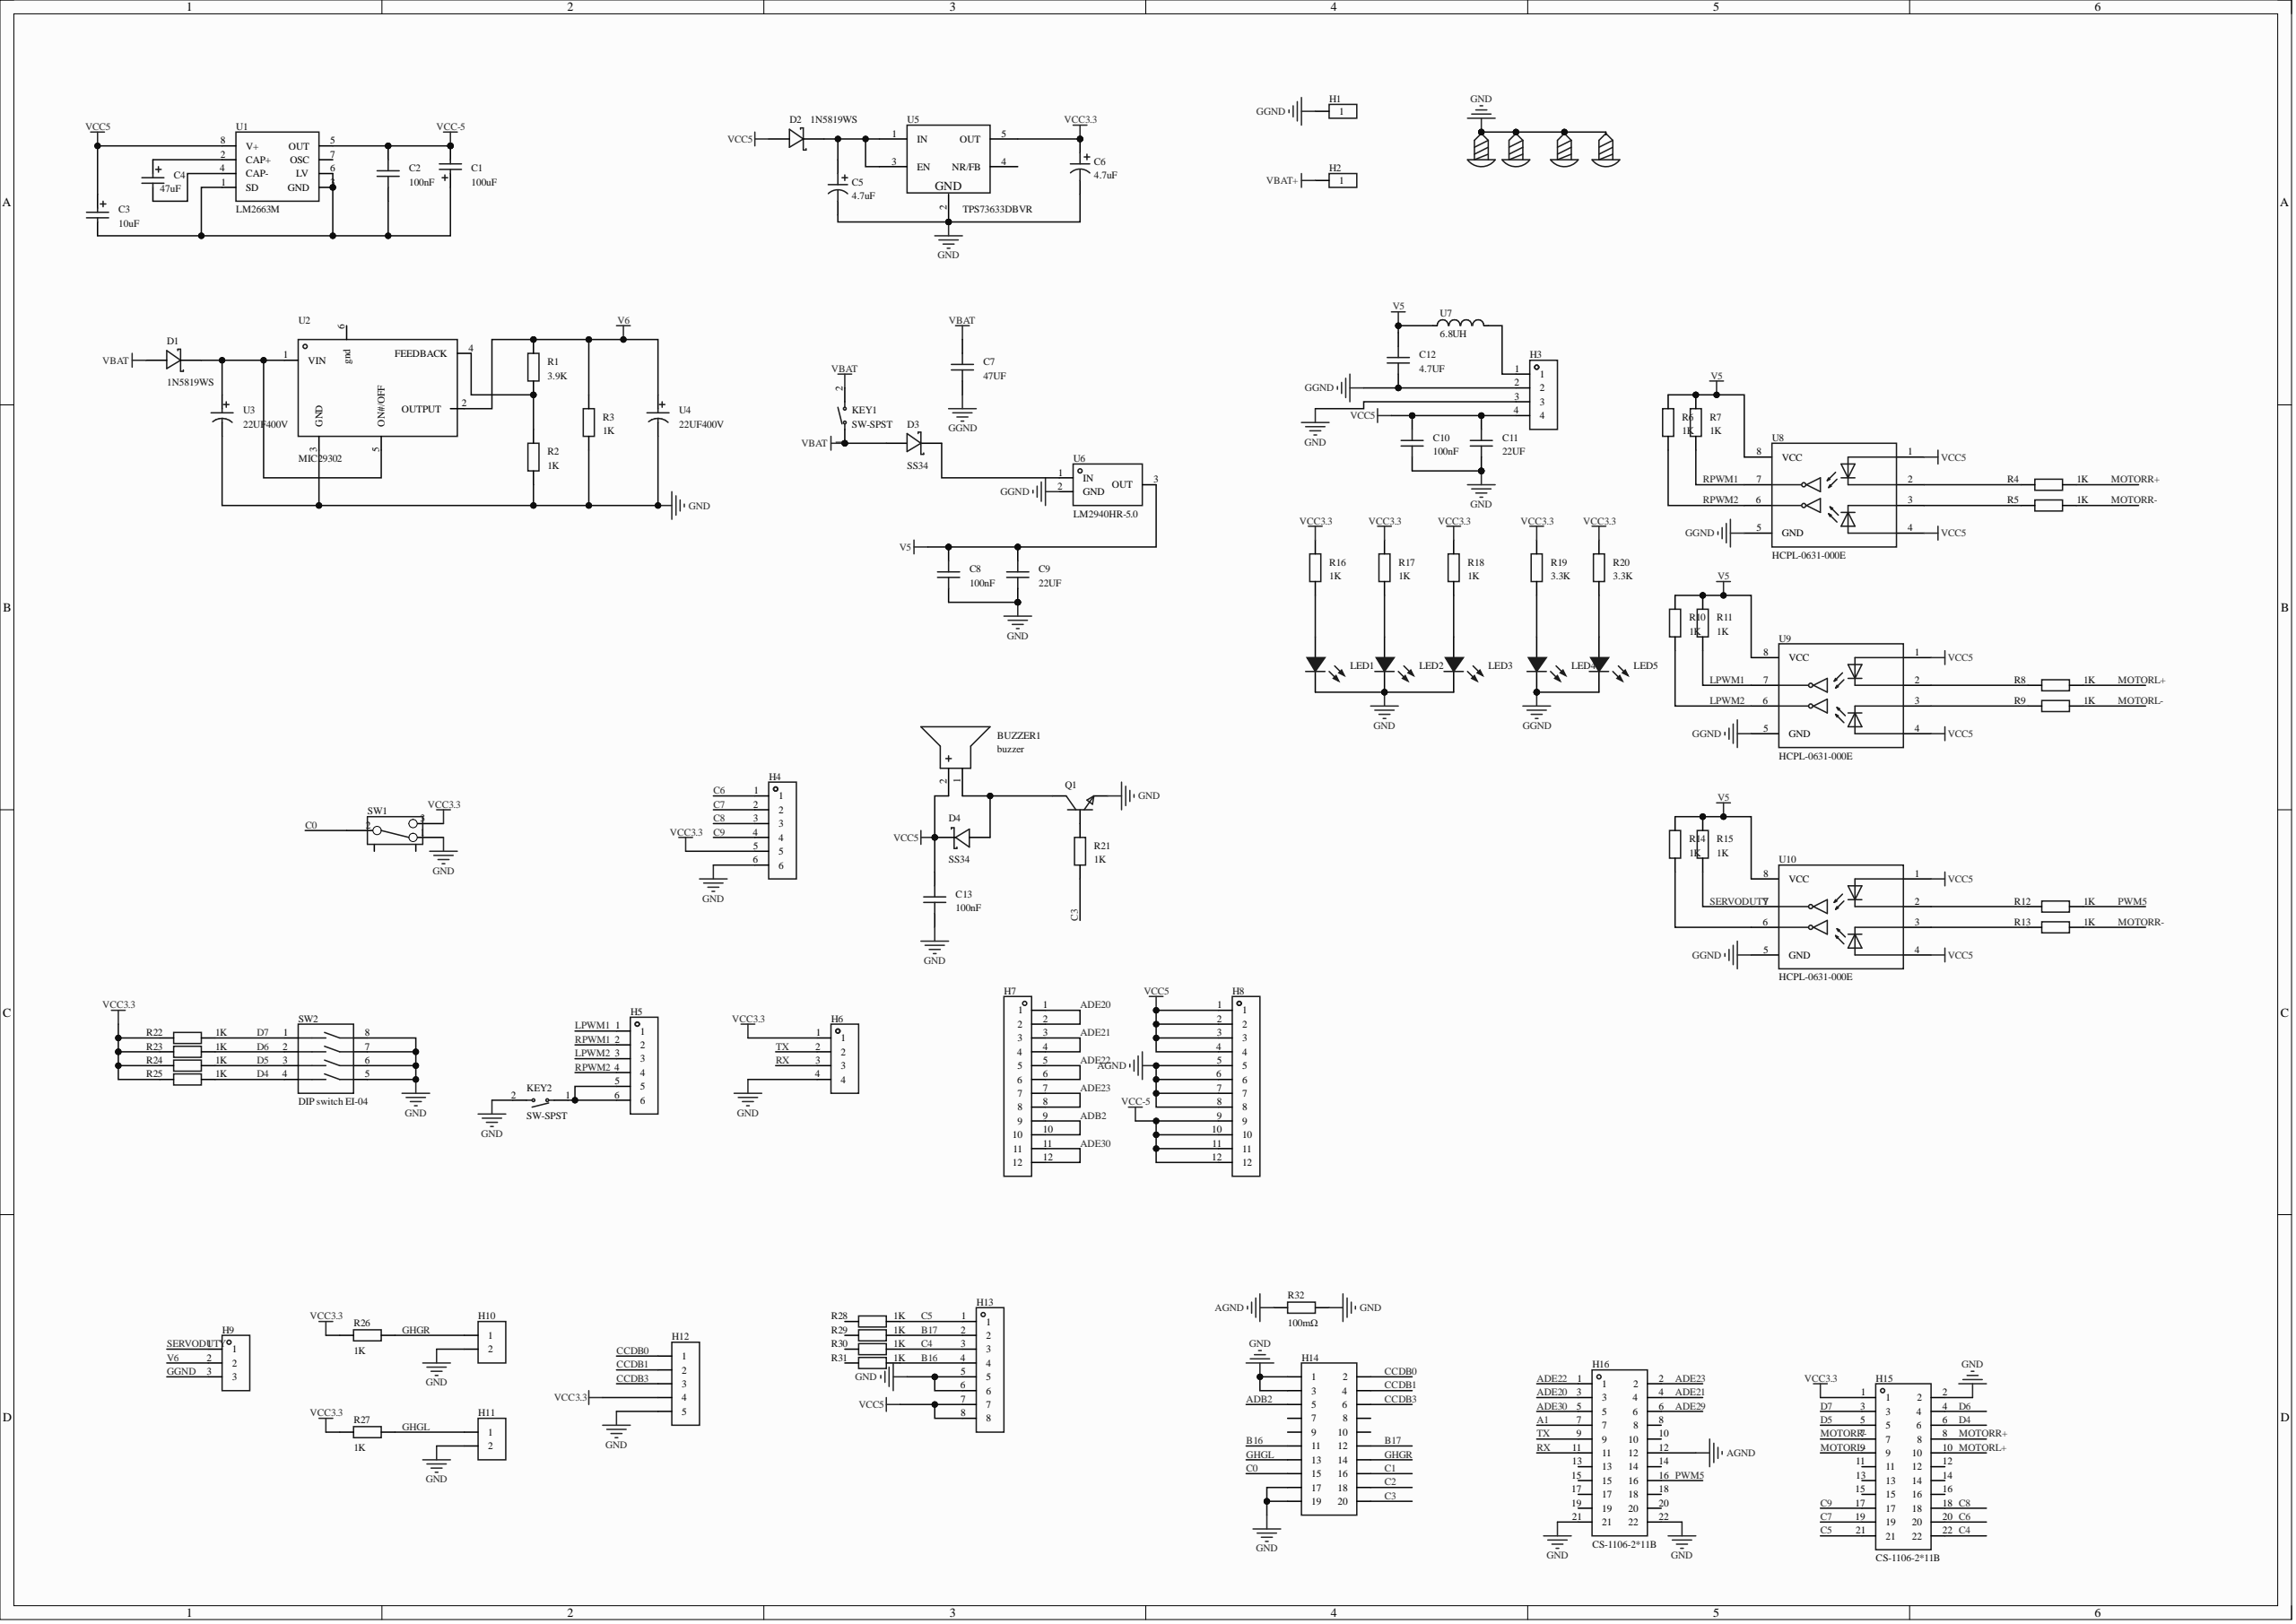Circuit board | Altium Designer | 90 parts | 69 nets
Bill of materials:
Comment,Description,Designator,Footprint,LibRef,Quantity
"buzzer","","BUZZER1","BUZ-TH_BD12.0-P6.00-D0.9-RD","buzzer","1"
"100uF","","C1","C_Ele_SMD_3x5.4mm","C_Ele_SMD_3x5.4mm","1"
"100nF","","C2, C8, C10, C13","C0603","CAP_0603","4"
"10uF","","C3","C_Ele_SMD_3x5.4mm","C_Ele_SMD_3x5.4mm","1"
"47uF","","C4","C_Ele_SMD_3x5.4mm","C_Ele_SMD_3x5.4mm","1"
"4.7uF","Capacitance: 4.7uF; tolerance: ±20%; rated voltage: 400V; ripple current: 220mA@100KHz; equivalent series resistance (ESR): 11Ω;","C5, C6","CAP-TH_BD8.0-P3.50-D0.5-FD_4.7UF400V8X14FS","4.7uF400V8x14FS","2"
"47UF","","C7","C1206","47UF","1"
"22UF","","C9, C11","C1206","22UF","2"
"4.7UF","","C12","C0603","CAP_0603","1"
"1N5819WS","Forward voltage (Vf): 600mV@1A; DC reverse voltage (Vr): 40V; rectified current: 1A;","D1, D2","SOD-323_L1.8-W1.3-LS2.5-RD","1N5819WS_C191023","2"
"SS34","Diode configuration: single; forward voltage (Vf): 550mV@3A; DC reverse voltage (Vr): 40V; rectified current: 3A;","D3","SMA_L4.3-W2.6-LS5.2-RD","SS34_C8678","1"
"SS34","","D4","SMA_L4.3-W2.6-LS5.0-RD","SS34","1"
"","","H1, H2","HDR-TH_1P-V-M_XKB_X4611WV-01I-C28D40","HDR-M_2.54_1x1P","2"
"","","H3, H6","HDR-TH_4P-P2.54-V-F","HDR-F_2.54_1x4P","2"
"","","H4, H5","HDR-TH_6P-P2.54-V-F","HDR-F_2.54_1x6P","2"
"","","H7, H8","HDR-TH_12P-P2.54-V-F","HDR-F_2.54_1x12P","2"
"","","H9","HDR-TH_3P-P2.54-V-F","HDR-F_2.54_1x3P","1"
"","","H10, H11","HDR-TH_2P-P2.54-V-F","HDR-F_2.54_1x2P","2"
"","","H12","HDR-TH_5P-P2.54-V-F","HDR-F_2.54_1x5P","1"
"","","H13","HDR-TH_8P-P2.54-V-F-1","HDR-F_2.54_1x8P","1"
"","","H14","HDR-TH_20P-P2.54-V-R2-C10-S2.54","HDR-F_2.54_2x10","1"
"CS-1106-2*11B","","H15, H16","HDR-TH_22P-P2.54-V-M-R2-C11-S2.54-1","CS-1106-2*11B","2"
"SW-SPST","","KEY1, KEY2","KEY-SMD_L6.0-W3.6-LS8.0","SW-SPST-SMT3*6*2.5贴片按钮","2"
"","","LED1, LED2, LED3, LED4, LED5","LED-TH_5mm","LED_TH-B_5mm","5"
"","","Q1","S8050_TO_92","S8050_TO_NPN","1"
"3.9K","","R1","R0603","Res_0603","1"
"1K","","R2, R3, R4, R5, R6, R7, R8, R9, R10, R11, R12, R13, R14, R15, R16, R17, R18, R21, R22, R23, R24, R25, R26, R27, R28, R29, R30, R31","R0603","Res_0603","28"
"3.3K","","R19, R20","R0603","Res_0603","2"
"100mΩ","Resistor type: thick film resistor; resistance: 100mΩ; tolerance: ±1%; power: 250mW; operating voltage: 200V; temperature coefficient: ±800ppm/?;","R32","R1206","1206W4F100LT5E","1"
"","","SCREW1, SCREW2, SCREW3, SCREW4","M2螺丝","M2螺丝","4"
"","","SW1","拨动开关","拨动开关_正","1"
"DIP switch EI-04","Type: flat lever, raised; circuit structure: SPST; switch positions: 4; service life: -; colour: black;","SW2","SW-TH_DIPSWITCHEI-04","拨码开关EI-04","1"
"LM2663M","LM2663 200mA switched-capacitor voltage converter with low-current shutdown mode","U1","SOIC-8_L4.9-W3.9-P1.27-LS6.0-BL","LM2663M","1"
"MIC29302","","U2","TO-263-5_L10.1-W8.7-P1.70-LS15.2-BR","MIC29302","1"
"22UF400V","","U3, U4","CAP-TH_BD8.0-P3.50-D0.6-FD","22UF400V","2"
"TPS73633DBVR","Output type: fixed; max input voltage: 5.5V; output voltage: 3.3V; output current: 400mA; PSRR: 58dB@(100Hz); 37dB@(10kHz); output polarity: positive;","U5","SOT-23-5_L3.0-W1.7-P0.95-LS2.8-BR","TPS73633DBVR","1"
"LM2940HR-5.0","","U6","TO-263-2_L10.1-W9.1-P5.08-LS15.2-BR","LM2940HR-5.0","1"
"6.8UH","","U7","IND-SMD_L10.9-W10.0_ACL1009","6.8UH","1"
"HCPL-0631-000E","Input type: DC; operating voltage: 4.5V~5.5V; data rate: 10Mbps;","U8, U9, U10","SO-8_L5.1-W3.9-P1.27-LS6.0-BL","HCPL-0631-000E","3"
Netlist (Protel format):
[
BUZZER1
BUZ-TH_BD12.0-P6.00-D0.9-RD
buzzer



]
[
C1
C_Ele_SMD_3x5.4mm
100uF



]
[
C2
C0603
100nF



]
[
C3
C_Ele_SMD_3x5.4mm
10uF



]
[
C4
C_Ele_SMD_3x5.4mm
47uF



]
[
C5
CAP-TH_BD8.0-P3.50-D0.5-FD_4.7UF400V8X14FS
4.7uF



]
[
C6
CAP-TH_BD8.0-P3.50-D0.5-FD_4.7UF400V8X14FS
4.7uF



]
[
C7
C1206
47UF



]
[
C8
C0603
100nF



]
[
C9
C1206
22UF



]
[
C10
C0603
100nF



]
[
C11
C1206
22UF



]
[
C12
C0603
4.7UF



]
[
C13
C0603
100nF



]
[
D1
SOD-323_L1.8-W1.3-LS2.5-RD
1N5819WS



]
[
D2
SOD-323_L1.8-W1.3-LS2.5-RD
1N5819WS



]
[
D3
SMA_L4.3-W2.6-LS5.2-RD
SS34



]
[
D4
SMA_L4.3-W2.6-LS5.0-RD
SS34



]
[
H1
HDR-TH_1P-V-M_XKB_X4611WV-01I-C28D40




]
[
H2
HDR-TH_1P-V-M_XKB_X4611WV-01I-C28D40




]
[
H3
HDR-TH_4P-P2.54-V-F




]
[
H4
HDR-TH_6P-P2.54-V-F




]
[
H5
HDR-TH_6P-P2.54-V-F




]
[
H6
HDR-TH_4P-P2.54-V-F




]
[
H7
HDR-TH_12P-P2.54-V-F




]
[
H8
HDR-TH_12P-P2.54-V-F




]
[
H9
HDR-TH_3P-P2.54-V-F




]
[
H10
HDR-TH_2P-P2.54-V-F




]
[
H11
HDR-TH_2P-P2.54-V-F




]
[
H12
HDR-TH_5P-P2.54-V-F




]
[
H13
HDR-TH_8P-P2.54-V-F-1




]
[
H14
HDR-TH_20P-P2.54-V-R2-C10-S2.54




]
[
H15
HDR-TH_22P-P2.54-V-M-R2-C11-S2.54-1
CS-1106-2*11B



]
[
H16
HDR-TH_22P-P2.54-V-M-R2-C11-S2.54-1
CS-1106-2*11B



]
[
KEY1
KEY-SMD_L6.0-W3.6-LS8.0
SW-SPST



]
[
KEY2
KEY-SMD_L6.0-W3.6-LS8.0
SW-SPST



]
[
LED1
LED-TH_5mm




]
[
LED2
LED-TH_5mm




]
[
LED3
LED-TH_5mm




]
[
LED4
LED-TH_5mm




]
[
LED5
LED-TH_5mm




]
[
Q1
S8050_TO_92




]
[
R1
R0603
3.9K



]
[
R2
R0603
1K



]
[
R3
R0603
1K



]
[
R4
R0603
1K



]
[
R5
R0603
1K



]
[
R6
R0603
1K



]
[
R7
R0603
1K



]
[
R8
R0603
1K



]
[
R9
R0603
1K



]
[
R10
R0603
1K



]
[
R11
R0603
1K



]
[
R12
R0603
1K



]
[
R13
R0603
1K



]
[
R14
R0603
1K



]
[
R15
R0603
1K



]
[
R16
R0603
1K



]
[
R17
R0603
1K



]
[
R18
R0603
1K



]
[
R19
R0603
3.3K



]
[
R20
R0603
3.3K



]
[
R21
R0603
1K



]
[
R22
R0603
1K



]
[
R23
R0603
1K



]
[
R24
R0603
1K



]
[
R25
R0603
1K



]
[
R26
R0603
1K



]
[
R27
R0603
1K



]
[
R28
R0603
1K



]
[
R29
R0603
1K



]
[
R30
R0603
1K



]
[
R31
R0603
1K



]
[
R32
R1206
100mΩ



]
[
SCREW1
M2螺丝




]
[
SCREW2
M2螺丝




]
[
SCREW3
M2螺丝




]
[
SCREW4
M2螺丝




]
[
SW1
拨动开关




]
[
SW2
SW-TH_DIPSWITCHEI-04
DIP switch EI-04



]
[
U1
SOIC-8_L4.9-W3.9-P1.27-LS6.0-BL
LM2663M



]
[
U2
TO-263-5_L10.1-W8.7-P1.70-LS15.2-BR
MIC29302



]
[
U3
CAP-TH_BD8.0-P3.50-D0.6-FD
22UF400V



]
[
U4
CAP-TH_BD8.0-P3.50-D0.6-FD
22UF400V



]
[
U5
SOT-23-5_L3.0-W1.7-P0.95-LS2.8-BR
TPS73633DBVR



]
[
U6
TO-263-2_L10.1-W9.1-P5.08-LS15.2-BR
LM2940HR-5.0



]
[
U7
IND-SMD_L10.9-W10.0_ACL1009
6.8UH



]
[
U8
SO-8_L5.1-W3.9-P1.27-LS6.0-BL
HCPL-0631-000E



]
[
U9
SO-8_L5.1-W3.9-P1.27-LS6.0-BL
HCPL-0631-000E



]
[
U10
SO-8_L5.1-W3.9-P1.27-LS6.0-BL
HCPL-0631-000E



]
(
VCC-5
C1-2
C2-2
H8-9
H8-10
H8-11
H8-12
U1-5
)
(
VCC5
BUZZER1-2
C3-1
C10-2
C11-2
C13-2
D2-2
D4-1
H3-4
H8-1
H8-2
H8-3
H8-4
H13-7
H13-8
U1-8
U8-1
U8-4
U9-1
U9-4
U10-1
U10-4
)
(
VCC3.3
C6-1
H4-5
H6-1
H12-4
H15-1
R16-2
R17-2
R18-2
R19-2
R20-2
R22-1
R23-1
R24-1
R25-1
R26-1
R27-1
SW1-3
U5-5
)
(
VBAT
C7-1
D1-2
D3-2
KEY1-1
KEY1-2
)
(
V6
H9-2
R1-2
R3-2
U2-2
U4-1
)
(
V5
C8-2
C9-2
C12-2
R6-2
R7-2
R10-2
R11-2
R14-2
R15-2
U6-3
U7-1
U8-8
U9-8
U10-8
)
(
TX
H6-2
H16-9
)
(
SERVODUTY
H9-1
R15-1
U10-7
)
(
RX
H6-3
H16-11
)
(
RPWM2
H5-4
R6-1
U8-6
)
(
RPWM1
H5-2
R7-1
U8-7
)
(
PWM5
H16-16
R12-2
)
(
NetR14_1
R14-1
U10-6
)
(
NetR13_1
R13-1
U10-3
)
(
NetR12_1
R12-1
U10-2
)
(
NetR9_1
R9-1
U9-3
)
(
NetR8_1
R8-1
U9-2
)
(
NetR5_1
R5-1
U8-3
)
(
NetR4_1
R4-1
U8-2
)
(
NetR1_1
R1-1
R2-2
U2-4
)
(
NetQ1_2
Q1-2
R21-2
)
(
NetLED5_1
LED5-1
R20-1
)
(
NetLED4_1
LED4-1
R19-1
)
(
NetLED3_1
LED3-1
R18-1
)
(
NetLED2_1
LED2-1
R17-1
)
(
NetLED1_1
LED1-1
R16-1
)
(
NetH5_5
H5-5
H5-6
KEY2-1
)
(
NetH3_1
H3-1
U7-2
)
(
NetD3_1
D3-1
U6-1
)
(
NetD1_1
D1-1
U2-1
U2-5
U3-1
)
(
NetC5_1
C5-1
D2-1
U5-1
U5-3
)
(
NetC4_2
C4-2
U1-4
)
(
NetC4_1
C4-1
U1-2
)
(
NetC1_1
C1-1
C2-1
C3-2
U1-1
U1-3
U1-6
)
(
NetBUZZER1_1
BUZZER1-1
D4-2
Q1-3
)
(
MOTORR-
H15-7
R5-2
R13-2
)
(
MOTORR+
H15-8
R4-2
)
(
MOTORL-
H15-9
R9-2
)
(
MOTORL+
H15-10
R8-2
)
(
LPWM2
H5-3
R10-1
U9-6
)
(
LPWM1
H5-1
R11-1
U9-7
)
(
GND
C5-2
C6-2
C8-1
C9-1
C10-1
C11-1
C13-1
H3-3
H4-6
H6-4
H10-2
H11-2
H12-5
H13-5
H13-6
H14-1
H14-3
H14-17
H14-19
H15-2
H16-21
H16-22
KEY2-2
LED1-2
LED2-2
LED3-2
Q1-1
R2-1
R3-1
R32-2
SCREW1-1
SCREW2-1
SCREW3-1
SCREW4-1
SW1-1
SW2-5
SW2-6
SW2-7
SW2-8
U2-3
U3-2
U4-2
U5-2
)
(
GHGR
H10-1
H14-14
R26-2
)
(
GHGL
H11-1
H14-13
R27-2
)
(
GGND
C7-2
C12-1
H1-1
H3-2
H9-3
LED4-2
LED5-2
U6-2
U8-5
U9-5
U10-5
)
(
D7
H15-3
R22-2
SW2-1
)
(
D6
H15-4
R23-2
SW2-2
)
(
D5
H15-5
R24-2
SW2-3
)
(
D4
H15-6
R25-2
SW2-4
)
(
CCDB3
H12-3
H14-6
)
(
CCDB1
H12-2
H14-4
)
(
CCDB0
H12-1
H14-2
)
(
C9
H4-4
H15-17
)
(
C8
H4-3
H15-18
)
(
C7
H4-2
H15-19
)
(
C6
H4-1
H15-20
)
(
C5
H13-1
H15-21
R28-2
)
(
C4
H13-3
H15-22
R30-2
)
(
C3
H14-20
R21-1
)
(
C0
H14-15
SW1-2
)
(
B17
H13-2
H14-12
R29-2
)
(
B16
H13-4
H14-11
R31-2
)
(
AGND
H8-5
H8-6
H8-7
H8-8
H16-12
R32-1
)
(
ADE30
H7-11
H7-12
H16-5
)
(
ADE23
H7-7
H7-8
H16-2
)
(
ADE22
H7-5
H7-6
H16-1
)
(
ADE21
H7-3
H7-4
H16-4
)
(
ADE20
H7-1
H7-2
H16-3
)
(
ADB2
H7-9
H7-10
H14-5
)